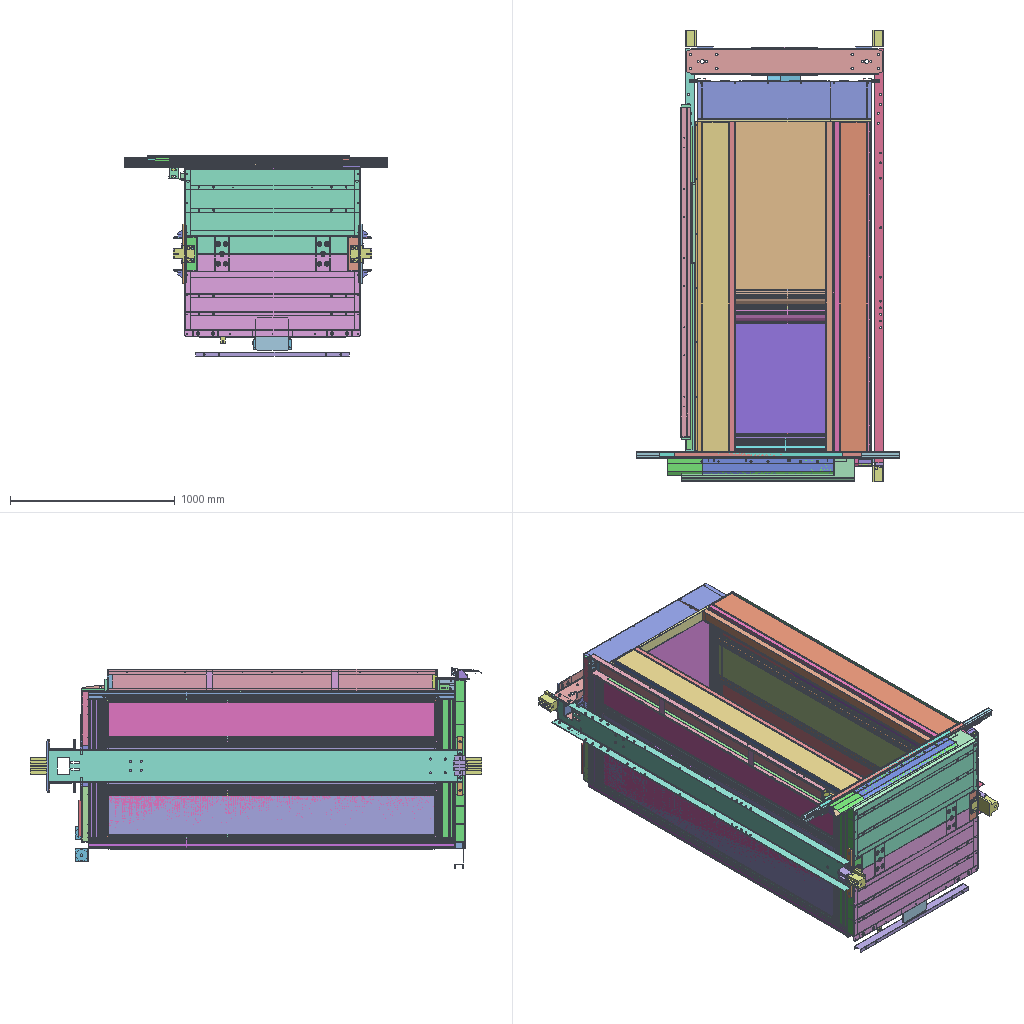Assembly | SolidWorks | 198 different items | 343 placed | box 1600 x 2739 x 1215 mm
Parts list (item | name | quantity | parent item):
1 | 25-2905 25-220S   常规梯专用电缆板A | x1 | in 145
2 | 25-2905 25-220S   轿顶简易盖板 | x1 | in 145
3 | 25-2905 25-220S   轿顶装饰板前 | x2 | in 145
4 | 25-2905 25-220S   轿顶装饰板后 | x2 | in 145
5 | 25-2905 25-220S  70地坎支架 | x1 | in 29
6 | 25-2905 25-220S  70地坎支架筋板 | x4 | in 29
7 | 25-2905 25-220S  L型支架 | x12 | in 135
8 | 25-2905 25-220S  U型支架 | x4 | in 131
9 | 25-2905 25-220S  歌拉瑞70旁开门地坎支架 | x1 | in 10
10 | 25-2905 25-220S  歌拉瑞70旁开门地坎支架焊件 (subassembly) | x1 | in 124
11 | 25-2905 25-220S  歌拉瑞70旁开门地坎支架筋板 | x4 | in 10
12 | 25-2905 25-220S  称重板 | x1 | in 142
13 | 25-2905 25-220S  背玻璃框（栅格板）（含扶手版） | x1 | in 135
14 | 25-2905 25-220S  轿底电缆固定板 | x1 | in 142
15 | 25-2905 25-220S  铝合金地坎(更新） | x1 | in 137
16 | 25-2905 25-220S 40地坎支架 | x1 | in 18
17 | 25-2905 25-220S 40地坎支架加筋 | x6 | in 18
18 | 25-2905 25-220S 40地坎支架焊件 (subassembly) | x1 | in 19
19 | 25-2905 25-220S 40地坎组件 (subassembly) | x1 | in 102
20 | 25-2905 25-220S 40护脚板 | x1 | in 19
21 | 25-2905 25-220S 40铝合金地坎 | x1 | in 19
22 | 25-2905 25-220S 60地坎护脚板 | x1 | in 26
23 | 25-2905 25-220S 60地坎支架 | x1 | in 24
24 | 25-2905 25-220S 60地坎支架焊件 (subassembly) | x1 | in 26
25 | 25-2905 25-220S 60地坎支架筋板 | x4 | in 24
26 | 25-2905 25-220S 60地坎支架组件 (subassembly) | x1 | in 102
27 | 25-2905 25-220S 60铝合金地坎 | x1 | in 26
28 | 25-2905 25-220S 70地坎(中分双折) | x1 | in 30
29 | 25-2905 25-220S 70地坎支架焊件(中分双折) (subassembly) | x1 | in 30
30 | 25-2905 25-220S 70地坎支架组件(中分双折) (subassembly) | x1 | in 102
31 | 25-2905 25-220S 70护脚板(中分双折) | x1 | in 30
32 | 25-2905 25-220S DD  吊顶 (subassembly) | x1 | in 137
33 | 25-2905 25-220S DD  外协吊顶 | x1 | in 32
34 | 25-2905 25-220S DD  星空顶A主板 | x1 | in 38
35 | 25-2905 25-220S DD  星空顶A客户确认图 (subassembly) | x1 | in 32
36 | 25-2905 25-220S DD  星空顶A封板 | x1 | in 38
37 | 25-2905 25-220S DD  星空顶A灯条框 | x1 | in 35
38 | 25-2905 25-220S DD  星空顶A焊件 (subassembly) | x1 | in 35
39 | 25-2905 25-220S DD  琉璃顶-内板 | x1 | in 42
40 | 25-2905 25-220S DD  琉璃顶-客户确认图 (subassembly) | x1 | in 32
41 | 25-2905 25-220S DD  琉璃顶-扩散板 | x1 | in 42
42 | 25-2905 25-220S DD  琉璃顶-灯罩框架 (subassembly) | x1 | in 40
43 | 25-2905 25-220S DD  琉璃顶-焊件总成 (subassembly) | x1 | in 40
44 | 25-2905 25-220S DD  琉璃顶-避让钣金 | x1 | in 43
45 | 25-2905 25-220S DD  琉璃顶-铝合金边框 | x1 | in 42
46 | 25-2905 25-220S DD  琉璃顶主板 | x1 | in 43
47 | 25-2905 25-220S DD  白顶-主板 | x1 | in 50
48 | 25-2905 25-220S DD  白顶-避让钣金 | x1 | in 50
49 | 25-2905 25-220S DD  白顶客户确认图 (subassembly) | x1 | in 32
50 | 25-2905 25-220S DD  白顶焊件总成 (subassembly) | x1 | in 49
51 | 25-2905 25-220S DD  白顶边框 | x1 | in 49
52 | 25-2905 25-220S DD-B1  白顶A主板 | x1 | in 56
53 | 25-2905 25-220S DD-B1  白顶A客户确认图 (subassembly) | x1 | in 32
54 | 25-2905 25-220S DD-B1  白顶A封板 | x1 | in 56
55 | 25-2905 25-220S DD-B1  白顶A灯条框 | x1 | in 53
56 | 25-2905 25-220S DD-B1  白顶A焊件 (subassembly) | x1 | in 53
57 | 25-2905 25-220S DD-X1  星空顶A主板 | x1 | in 61
58 | 25-2905 25-220S DD-X1  星空顶A客户确认图 (subassembly) | x1 | in 32
59 | 25-2905 25-220S DD-X1  星空顶A封板 | x1 | in 61
60 | 25-2905 25-220S DD-X1  星空顶A灯条框 | x1 | in 58
61 | 25-2905 25-220S DD-X1  星空顶A焊件 (subassembly) | x1 | in 58
62 | 25-2905 25-220S gyfb-75198(歌拉瑞专用风机) | x2 | in 137, 145
63 | 25-2905 25-220S 中立柱安装总成 (右侧） (subassembly) | x1 | in 131
64 | 25-2905 25-220S 中立柱安装总成 (左侧） (subassembly) | x1 | in 131
65 | 25-2905 25-220S 中间立柱COP外盖板 | x1 | in 64
66 | 25-2905 25-220S 中间立柱COP安装板 | x2 | in 64
67 | 25-2905 25-220S 中间立柱背板  (右侧） | x1 | in 63
68 | 25-2905 25-220S 中间立柱背板  (左侧） | x1 | in 64
69 | 25-2905 25-220S 中间立柱面板 (右侧） | x1 | in 63
70 | 25-2905 25-220S 中间立柱面板 (左侧） | x1 | in 64
71 | 25-2905 25-220S 侧前玻璃框 | x2 | in 135
72 | 25-2905 25-220S 侧后玻璃框 | x2 | in 135
73 | 25-2905 25-220S 侧玻璃框（HCS511) | x1 | in 135
74 | 25-2905 25-220S 侧筋板 | x22 | in 142
75 | 25-2905 25-220S 前壁右操纵箱加筋上（HOP029） | x1 | in 96
76 | 25-2905 25-220S 前壁右操纵箱加筋下（HOP029） | x1 | in 96
77 | 25-2905 25-220S 前壁左操纵箱加筋上（HOP029） | x1 | in 112
78 | 25-2905 25-220S 前壁左操纵箱加筋下（HOP029） | x1 | in 112
79 | 25-2905 25-220S 前壁操纵箱安装板（HOP029） | x2 | in 96, 112
80 | 25-2905 25-220S 反折DD-B1  白顶A主板 | x1 | in 82
81 | 25-2905 25-220S 反折DD-B1  白顶A封板 | x1 | in 82
82 | 25-2905 25-220S 反折DD-B1  白顶A焊件 (subassembly) | x1 | in 53
83 | 25-2905 25-220S 反折DD-X1  星空顶A主板 | x1 | in 85
84 | 25-2905 25-220S 反折DD-X1  星空顶A封板 | x1 | in 85
85 | 25-2905 25-220S 反折DD-X1  星空顶A焊件 (subassembly) | x1 | in 58
86 | 25-2905 25-220S 台阶螺钉 | x24 | in 63, 64
87 | 25-2905 25-220S 右前壁一体操纵箱 | x1 | in 137
88 | 25-2905 25-220S 右前壁下安装板 | x1 | in 93
89 | 25-2905 25-220S 右前壁主板 | x1 | in 93
90 | 25-2905 25-220S 右前壁常规加筋 | x1 | in 96
91 | 25-2905 25-220S 右前壁操纵箱加筋 | x2 | in 96
92 | 25-2905 25-220S 右前壁操纵箱加筋A | x1 | in 96
93 | 25-2905 25-220S 右前壁焊件 (subassembly) | x1 | in 96
94 | 25-2905 25-220S 右前壁盖板 | x1 | in 96
95 | 25-2905 25-220S 右前壁盖板（齐平盖板） | x1 | in 96
96 | 25-2905 25-220S 右前壁组件 (subassembly) | x1 | in 136
97 | 25-2905 25-220S 后玻璃框 | x1 | in 135
98 | 25-2905 25-220S 后筋板 | x6 | in 142
99 | 25-2905 25-220S 圆弧底板 | x2 | in 101
100 | 25-2905 25-220S 圆弧盖板 | x2 | in 101
101 | 25-2905 25-220S 圆弧盖板装配体 (subassembly) | x2 | in 135
102 | 25-2905 25-220S 地坎综合 (subassembly) | x1 | in 137
103 | 25-2905 25-220S 左前壁一体操纵箱 | x1 | in 137
104 | 25-2905 25-220S 左前壁下安装板 | x1 | in 109
105 | 25-2905 25-220S 左前壁主板 | x1 | in 109
106 | 25-2905 25-220S 左前壁常规加筋 | x1 | in 112
107 | 25-2905 25-220S 左前壁操纵箱加筋 | x2 | in 112
108 | 25-2905 25-220S 左前壁操纵箱加筋A | x1 | in 112
109 | 25-2905 25-220S 左前壁焊件 (subassembly) | x1 | in 112
110 | 25-2905 25-220S 左前壁盖板 | x1 | in 112
111 | 25-2905 25-220S 左前壁盖板（齐平盖板） | x1 | in 112
112 | 25-2905 25-220S 左前壁组件 (subassembly) | x1 | in 136
113 | 25-2905 25-220S 旁开门前壁主板 | x1 | in 117
114 | 25-2905 25-220S 旁开门前壁加筋 | x2 | in 117
115 | 25-2905 25-220S 旁开门前壁垫板 | x2 | in 118
116 | 25-2905 25-220S 旁开门前壁安装板 | x1 | in 117
117 | 25-2905 25-220S 旁开门前壁焊件 (subassembly) | x1 | in 118
118 | 25-2905 25-220S 旁开门前壁组件 (subassembly) | x1 | in 137
119 | 25-2905 25-220S 标准LOGO踏板 | x1 | in 137
120 | 25-2905 25-220S 横向加筋 | x2 | in 147
121 | 25-2905 25-220S 歌拉瑞-COP   (HOP027) | x3 | in 64, 96, 112
122 | 25-2905 25-220S 歌拉瑞-COP   (HOP029) | x3 | in 64, 96, 112
123 | 25-2905 25-220S 歌拉瑞70旁开门地坎 | x1 | in 124
124 | 25-2905 25-220S 歌拉瑞70旁开门地坎组件 (subassembly) | x1 | in 102
125 | 25-2905 25-220S 歌拉瑞70旁开门护脚板 | x1 | in 124
126 | 25-2905 25-220S 磁栅尺支架 | x2 | in 147
127 | 25-2905 25-220S 立柱面板加强型材 | x4 | in 63, 64
128 | 25-2905 25-220S 纵向加筋 | x2 | in 147
129 | 25-2905 25-220S 背玻璃框后壁扶手 | x1 | in 135
130 | 25-2905 25-220S 轿厢中立柱型材 | x4 | in 131
131 | 25-2905 25-220S 轿厢中立柱总成 (subassembly) | x1 | in 135
132 | 25-2905 25-220S 轿厢中立柱灯带 | x4 | in 131
133 | 25-2905 25-220S 轿厢中立柱灯带盖板 | x4 | in 131
134 | 25-2905 25-220S 轿厢型材框架 | x1 | in 135
135 | 25-2905 25-220S 轿厢型材框架A (subassembly) | x1 | in 136
136 | 25-2905 25-220S 轿厢总成 (subassembly) | x1 | in 137
137 | 25-2905 25-220S 轿厢总成A (subassembly) | x1 | -
138 | 25-2905 25-220S 轿底两侧加强筋 | x1 | in 142
139 | 25-2905 25-220S 轿底主板 | x1 | in 142
140 | 25-2905 25-220S 轿底加筋 | x6 | in 142
141 | 25-2905 25-220S 轿底横向加强筋 | x1 | in 142
142 | 25-2905 25-220S 轿底焊接总成 (subassembly) | x1 | in 143
143 | 25-2905 25-220S 轿底装配总成 (subassembly) | x1 | in 136
144 | 25-2905 25-220S 轿顶主板 | x1 | in 147
145 | 25-2905 25-220S 轿顶安装总成 (subassembly) | x1 | in 136
146 | 25-2905 25-220S 轿顶横向边梁 | x1 | in 147
147 | 25-2905 25-220S 轿顶焊接总成 (subassembly) | x1 | in 145
148 | 25-2905 25-220S 轿顶纵向边梁 | x1 | in 147
149 | 25-2905 25-220S 轿顶防晃支架 | x2 | in 147
150 | 25-2905 25-220S 门机支架 | x2 | in 147
151 | 25-2905 25-220S 门机支架A | x1 | in 147
152 | 25-2905 25-220S 门楣主板 | x1 | in 156
153 | 25-2905 25-220S 门楣加筋 | x1 | in 156
154 | 25-2905 25-220S 门楣加筋（门机门楣安装） | x1 | in 156
155 | 25-2905 25-220S 门楣安装件 (subassembly) | x1 | in 136
156 | 25-2905 25-220S 门楣焊件 (subassembly) | x1 | in 155
157 | 25-2905 25-220S 门楣盖板 | x1 | in 155
158 | 25-2905 25-220S 非标加筋中横 | x2 | in 147
159 | 25-2905 25-220S 非标加筋侧横 | x4 | in 147
160 | 25-2905 25-220S 非标加筋竖 | x2 | in 147
161 | 25-2905 25-220S-G 侧筋板A | x4 | in 171
162 | 25-2905 25-220S-G 侧筋板B | x1 | -
163 | 25-2905 25-220S-G 后筋板 | x6 | in 171
164 | 25-2905 25-220S-G 轿底两侧加强筋 | x1 | in 171
165 | 25-2905 25-220S-G 轿底中间加筋A | x2 | in 171
166 | 25-2905 25-220S-G 轿底中间加筋B | x4 | in 171
167 | 25-2905 25-220S-G 轿底主板 | x1 | in 171
168 | 25-2905 25-220S-G 轿底安装孔内加厚板 | x2 | in 171
169 | 25-2905 25-220S-G 轿底安装总成 (subassembly) | x1 | in 136
170 | 25-2905 25-220S-G 轿底横向加强筋 | x1 | in 171
171 | 25-2905 25-220S-G 轿底焊接总成 (subassembly) | x1 | in 169
172 | 25-2905 25-220S-G 轿底盖板 | x1 | in 169
173 | 25-2905 25-220S-G 轿底缓冲器加筋 | x2 | in 171
174 | 25-2905 GEH160 梁总成 (subassembly) | x1 | -
175 | 25-2905 GEH160上梁主板（3A646) | x2 | in 176
176 | 25-2905 GEH160上梁装配（3A654) (subassembly) | x1 | in 174
177 | 25-2905 GEH160导靴板（3A277) | x2 | in 176
178 | 25-2905 GEH160立梁主板（3B389) | x1 | in 182
179 | 25-2905 GEH160立梁安装板（3B384) | x1 | in 182
180 | 25-2905 GEH160立梁绳头上板（3B288) | x1 | in 176
181 | 25-2905 GEH160立梁绳头座（3B289) | x1 | in 176
182 | 25-2905 GEH160立梁装配（3B387) (subassembly) | x1 | in 174
183 | 25-2905 减震垫（BB011) | x1 | -
184 | 25-2905 外购A-1 电梯防晃卡板 | x4 | -
185 | 25-2905 导靴 | x2 | in 182, 198
186 | 25-2905 歌拉瑞 3Z159001导靴 | x4 | in 174
187 | 25-2905 镜向25-220S 侧玻璃框（HCS511) | x1 | in 135
188 | 25-2905 镜向25-220S 右前壁下安装板 | x1 | in 93
189 | 25-2905 镜向25-220S 左前壁下安装板 | x1 | in 109
190 | 25-2905 镜向25-220S 旁开门前壁安装板 | x1 | in 117
191 | 25-2905 镜向25-220S 轿底两侧加强筋 | x1 | in 142
192 | 25-2905 镜向25-220S 轿顶纵向边梁 | x1 | in 147
193 | 25-2905 镜向25-220S 门楣加筋 | x1 | in 156
194 | 25-2905 镜向25-220S-G 轿底两侧加强筋 | x1 | in 171
195 | hexagon weld nuts gb | x1 | -
196 | 镜向25-2905 GEH160立梁主板（3B266) | x1 | in 198
197 | 镜向25-2905 GEH160立梁安装板（3B265) | x1 | in 198
198 | 镜向25-2905 GEH160立梁装配（3B262) (subassembly) | x1 | in 174
Mates (type | each side: item.copy, entity, surface, feature):
In the top assembly
Coincident | assembly face | assembly face
Concentric | assembly face | assembly face
Coincident | 174.1 plane | assembly plane | 3 times
Coincident | 137.1 plane | assembly plane | 2 times
Width | 179.1 face plane 基体-法兰1 | 179.1 face plane 基体-法兰1 | 167.1 face plane 基体-法兰1 | 194.1 face plane 25-2905 25-220S-G 轿底两侧加强筋_镜向
Coincident | 178.1 face plane 基体-法兰1 | 184.1 face plane 凸台-拉伸1 | 2 times
Coincident | 149.1 face plane 边线-法兰1 | 184.1 face plane 基体-法兰1
In subassembly 174
Coincident | 174.2 face | 174.2 face
Concentric | 174.2 face | 174.2 face
Coincident | 176.1 plane | 174.2 plane | 2 times
Coincident | 182.1 plane | 174.2 plane
Coincident | 175.1 face plane 边线-法兰1 | 174.2 plane
Coincident | 175.1 face plane 边线-法兰1 | 178.2 face plane 基体-法兰1
Coincident | 177.1 face plane 基体-法兰1 | 186.1 face plane 凸台-拉伸1
Coincident | 174.2 plane | 186.1 plane
DistanceDim | 186.1 face plane 切除-拉伸1 | 178.2 face plane 基体-法兰1
Coincident | 186.1 face plane 切除-拉伸1 | 186.2 face plane 切除-拉伸1 | 2 times
DistanceDim | 186.2 face plane 凸台-拉伸1 | 178.2 face plane 基体-法兰1
Coincident | 186.1 plane | 174.2 plane
DistanceDim | 175.1 face plane 基体-法兰1 | 178.2 face plane 基体-法兰1
In subassembly 176
Coincident | 176.2 face | 176.2 face
Concentric | 176.2 face | 176.2 face
Coincident | 175.2 plane | 176.2 plane
Coincident | 175.2 face plane 边线-法兰1 | 176.2 plane
DistanceDim | 175.3 face plane 基体-法兰1 | 175.2 face plane 基体-法兰1
Coincident | 175.2 face plane 边线-法兰1 | 177.2 face plane 基体-法兰1
Coincident | 177.2 plane | 176.2 plane
DistanceDim | 177.2 plane | 175.3 face plane 基体-法兰1
Coincident | 181.1 plane | 176.2 plane | 2 times
Coincident | 175.2 face plane 边线-法兰1 | 181.1 face plane 边线-法兰2
Coincident | 180.1 plane | 176.2 plane | 2 times
Coincident | 175.3 face plane 边线-法兰1 | 180.1 face plane 基体-法兰1
In subassembly 182
Coincident | 182.2 face | 182.2 face
Concentric | 182.2 face | 182.2 face
Coincident | 178.3 plane | 182.2 plane
Coincident | 178.3 face plane 基体-法兰1 | 182.2 plane | 2 times
Coincident | 178.3 face plane 基体-法兰1 | 179.2 face plane 基体-法兰1 | 2 times
Coincident | 179.2 plane | 182.2 plane
Coincident | 178.3 face plane 基体-法兰1 | 185.1 face plane 凸台-拉伸1
DistanceDim | 185.1 face plane 凸台-拉伸1 | 178.3 face plane 基体-法兰1
In subassembly 137
Coincident | 137.2 face | 137.2 face
Concentric | 137.2 face | 137.2 face
Coincident | 136.1 plane | 137.2 plane | 3 times
DistanceDim | 21.1 face plane 凸台-拉伸1 | 134.1 face plane 25型材 25型材小立柱（最新）(1)
Coincident | 134.1 plane | 102.1 plane
Coincident | 139.1 face plane 基体-法兰1 | 103.1 face plane 镜向1
Coincident | 139.1 face plane 基体-法兰1 | 87.1 face plane 凸台-拉伸3
Coincident | 134.1 face plane 25型材 25型材小立柱（最新）(1) | 119.1 face plane 凸台-拉伸1 | 2 times
Coincident | 134.1 plane | 119.1 plane
Coincident | 21.1 face plane 凸台-拉伸1 | 15.1 face plane 凸台-拉伸1
Coincident | 16.1 face plane 基体-法兰1 | 15.1 face plane 凸台-拉伸1
Coincident | 15.1 plane | 137.2 plane
Coincident | 144.1 face plane 基体-法兰1 | 62.1 face plane 凸台-拉伸1
DistanceDim | 134.1 face plane 25型材 25型材小立柱（最新）(1) | 16.1 face plane 基体-法兰1
Coincident | 134.1 face plane 25型材 25型材小立柱（最新）(1) | 113.1 face plane 基体-法兰1
Coincident | 134.1 face plane 25型材 25型材小立柱（最新）(1) | 87.1 face plane 凸台-拉伸2
Coincident | 134.1 face plane 25型材 25型材小立柱（最新）(1) | 87.1 face plane 凸台-拉伸1
Coincident | 134.1 face plane 25型材 25型材小立柱（最新）(1) | 103.1 face plane 凸台-拉伸2
Coincident | 134.1 face plane 25型材 25型材小立柱（最新）(1) | 103.1 face plane 凸台-拉伸1
DistanceDim | 33.1 face plane 凸台-拉伸1 | 134.1 face plane 25轿厢 GC505&506(1) | 2 times
Coincident | 144.1 face plane 基体-法兰1 | 33.1 face plane 凸台-拉伸1
In subassembly 136
Coincident | 136.2 face | 136.2 face
Concentric | 136.2 face | 136.2 face
Coincident | 135.1 plane | 136.2 plane | 3 times
Coincident | 145.1 plane | 136.2 plane | 2 times
Coincident | 134.2 face plane  D:\xxxxxx\xxxx\xxxx\xxxx\xxxx\xxxxxxxxxxxxx | 144.2 face plane 基体-法兰1
Coincident | 155.1 plane | 136.2 plane
Coincident | 144.2 face plane 边线-法兰2 | 152.1 face plane 边线-法兰5
Coincident | 143.1 plane | 136.2 plane | 2 times
Coincident | 134.2 face plane  D:\xxxxxx\xxxx\xxxx\xxxx\xxxx\xxxxxxxxxxxxx | 139.2 face plane 基体-法兰1
Coincident | 139.2 face plane 基体-法兰1 | 189.1 face plane 25-2905 25-220S 左前壁下安装板_镜向
Coincident | 171.1 plane | 136.2 plane
Coincident | 134.2 face plane 25轿厢 GC503(1) | 167.2 face plane 基体-法兰1
Coincident | 169.1 plane | 136.2 plane
Coincident | 134.2 face plane 25型材 25型材小立柱（最新）(1) | 88.1 face plane 基体-法兰1
Coincident | 134.2 face plane 25型材 25型材小立柱（最新）(1) | 152.1 face plane 基体-法兰1
Coincident | 134.2 face plane 25型材 25型材小立柱（最新）(1) | 105.1 face plane 基体-法兰1 | 2 times
Coincident | 134.2 face plane 25型材 25型材小立柱（最新）(1) | 89.1 face plane 基体-法兰1 | 2 times
In subassembly 135
Coincident | 135.2 face | 135.2 face
Concentric | 135.2 face | 135.2 face
Coincident | 134.3 plane | 135.2 plane | 3 times
Coincident | 131.1 plane | 135.2 plane | 2 times
Coincident | 134.3 face plane 25轿厢 GC503(1) | 130.1 face plane 凸台-拉伸1
Width | 7.1 face plane 基体-法兰1 | 7.1 face plane 基体-法兰1 | 134.3 face plane 25轿厢 GC503(1) | 134.3 face plane 25轿厢 GC503(1)
Coincident | 134.3 face plane 25轿厢 GC503(1) | 7.1 face plane 基体-法兰1
Coincident | 134.3 face plane  D:\xxxxxx\xxxx\xxxx\xxxx\xxxx\xxxxxxxxxxxxx | 7.1 face plane 基体-法兰1
Coincident | 134.3 face plane  D:\xxxxxx\xxxx\xxxx\xxxx\xxxx\xxxxxxxxxxxxx | 7.2 face plane 基体-法兰1
Parallel | 7.2 edge | 7.1 face plane 基体-法兰1
Coincident | 7.1 edge | 7.2 face plane 基体-法兰1
Coincident | 134.3 face plane 25轿厢 GC505&506(1) | 7.2 face plane 基体-法兰1
Coincident | 7.1 face plane 基体-法兰1 | 7.3 face plane 基体-法兰1
Coincident | 134.3 face plane  D:\xxxxxx\xxxx\xxxx\xxxx\xxxx\xxxxxxxxxxxxx | 7.3 face plane 基体-法兰1
Width | 7.3 face plane 基体-法兰1 | 7.3 face plane 基体-法兰1 | 134.3 face plane 25轿厢 GC503(1) | 134.3 face plane 25轿厢 GC503(1)
Coincident | 134.3 face plane 25轿厢 GC505&506(1) | 7.4 face plane 基体-法兰1
Coincident | 134.3 face plane  D:\xxxxxx\xxxx\xxxx\xxxx\xxxx\xxxxxxxxxxxxx | 7.4 face plane 基体-法兰1
Coincident | 7.3 face plane 基体-法兰1 | 7.4 edge
Coincident | 97.1 face plane  D:\xxxxxx\xx\xxxx\xxxx\xxxxxx\xxx\xxxxxxxxxxxx | 129.1 face plane  D:\xxxxxx\xx\xxxx\xxxx\xxxxxx\xxx\xxxxxxxxxxxx | 3 times
Coincident | 97.1 plane | 135.2 plane
Coincident | 134.3 face plane 25轿厢 GC503(1) | 97.1 face plane  D:\xxxxxx\xx\xxxx\xxxx\xxxxxx\xxx\xxxxxxxxxxxx | 2 times
Coincident | 134.3 face plane 25轿厢 GC503(1) | 72.1 face plane  D:\xxxxxx\xx\xxxx\xxxx\xxxxxx\xxx\xxxxxxxxxxxx | 2 times
Coincident | 134.3 face plane 25轿厢 GC503(1) | 73.1 face plane  D:\xxxxxx\xx\xxxx\xxxx\xxxxxx\xxx\xxxxxxxxxxxx | 2 times
Coincident | 134.3 face plane 25轿厢 GC503(1) | 71.1 face plane  D:\xxxxxx\xx\xxxx\xxxx\xxxxxx\xxx\xxxxxxxxxxxx | 2 times
DistanceDim | 134.3 edge | 72.1 face plane  D:\xxxxxx\xx\xxxx\xxxx\xxxxxx\xxx\xxxxxxxxxxxx
DistanceDim | 134.3 face plane  D:\xxxxxx\xxxx\xxxx\xxxx\xxxx\xxxxxxxxxxxxx | 73.1 face plane  D:\xxxxxx\xx\xxxx\xxxx\xxxxxx\xxx\xxxxxxxxxxxx
Coincident | 134.3 face plane  D:\xxxxxx\xxxx\xxxx\xxxx\xxxx\xxxxxxxxxxxxx | 99.1 face plane 凸台-拉伸1
Width | 99.1 face plane 凸台-拉伸1 | 99.1 face plane 凸台-拉伸1 | 134.3 face plane  D:\xxxxxx\xxxx\xxxx\xxxx\xxxx\xxxxxxxxxxxxx | 134.3 face plane  D:\xxxxxx\xxxx\xxxx\xxxx\xxxx\xxxxxxxxxxxxx
Coincident | 134.3 face plane  D:\xxxxxx\xxxx\xxxx\xxxx\xxxx\xxxxxxxxxxxxx | 100.1 face plane 凸台-拉伸1
DistanceDim | 130.1 face plane 凸台-拉伸1 | 71.1 edge
Coincident | 134.3 face plane 25轿厢 GC503(1) | 7.5 face plane 基体-法兰1
Coincident | 134.3 face plane 25型材 25型材小立柱（最新）(1) | 7.5 face plane 基体-法兰1
Coincident | 7.3 face plane 基体-法兰1 | 7.5 face plane 基体-法兰1
Coincident | 7.5 face plane 基体-法兰1 | 7.6 face plane 基体-法兰1 | 2 times
Coincident | 134.3 face plane 25轿厢 GC505&506(1) | 7.6 face plane 基体-法兰1
Coincident | 97.1 face plane  D:\xxxxxx\xx\xxxx\xxxx\xxxxxx\xxx\xxxxxxxxxxxx | 13.1 face plane  D:\xxxxxx\xx\xxxx\xxxx\xxxxxx\xxx\xxxxxxxxxxxx | 3 times
In subassembly 101
Coincident | 101.1 face | 101.1 face
Concentric | 101.1 face | 101.1 face
Coincident | 99.2 plane | 101.1 plane | 3 times
Coincident | 100.2 plane | 101.1 plane | 3 times
In subassembly 131
Coincident | 131.2 face | 131.2 face
Concentric | 131.2 face | 131.2 face
Parallel | 130.2 face plane 凸台-拉伸1 | 131.2 plane | 2 times
Coincident | 130.2 face plane 凸台-拉伸1 | 132.1 face plane 凸台-拉伸1 | 2 times
Coincident | 130.2 plane | 131.2 plane
Coincident | 132.1 plane | 131.2 plane
DistanceDim | 132.1 face plane 凸台-拉伸1 | 133.1 face plane 凸台-拉伸1
Coincident | 133.1 plane | 131.2 plane
Coincident | 132.1 face plane 凸台-拉伸1 | 133.1 edge
Coincident | 130.2 face plane 凸台-拉伸1 | 131.2 select_type:10 | 2 times
Coincident | 64.1 plane | 131.2 plane | 2 times
Coincident | 68.1 face plane 基体-法兰1 | 130.3 face plane 凸台-拉伸1
Coincident | 130.4 face plane 凸台-拉伸1 | 67.1 face plane 基体-法兰1
Coincident | 8.1 plane | 131.2 plane
DistanceDim | 68.1 face plane 基体-法兰1 | 8.1 face plane 基体-法兰1
DistanceDim | 8.1 face plane 基体-法兰1 | 130.3 face plane 凸台-拉伸1
Coincident | 8.2 plane | 131.2 plane
Coincident | 8.1 face plane 基体-法兰1 | 8.2 face plane 基体-法兰1
DistanceDim | 130.2 face plane 凸台-拉伸1 | 8.2 face plane 基体-法兰1
Coincident | 63.1 plane | 131.2 plane | 2 times
In subassembly 64
Coincident | 64.2 face | 64.2 face
Concentric | 64.2 face | 64.2 face
Coincident | 68.2 plane | 64.2 plane | 2 times
Coincident | 68.2 face plane 基体-法兰1 | 64.2 plane
Coincident | 70.1 plane | 64.2 plane | 2 times
Concentric | 68.2 face cylinder 切除-拉伸2 | 70.1 face cylinder 切除-拉伸2
Coincident | 70.1 face plane 基体-法兰1 | 66.1 face plane 基体-法兰1
Coincident | 70.1 plane | 66.1 plane
Coincident | 70.1 face plane 基体-法兰1 | 127.1 face plane 拉伸-薄壁1 | 2 times
Coincident | 127.1 plane | 64.2 plane
Concentric | 68.2 face cylinder 切除-拉伸2 | 86.1 face cylinder 凸台-拉伸3
Coincident | 68.2 face plane 基体-法兰1 | 86.1 face plane 凸台-拉伸2
Concentric | 68.2 face cylinder 切除-拉伸2 | 86.2 face cylinder 凸台-拉伸2
Coincident | 68.2 face plane 基体-法兰1 | 86.2 face plane 凸台-拉伸2
Concentric | 68.2 face cylinder 切除-拉伸2 | 86.3 face cylinder 凸台-拉伸2
Coincident | 68.2 face plane 基体-法兰1 | 86.3 face plane 凸台-拉伸2
Concentric | 68.2 face cylinder 切除-拉伸2 | 86.4 face cylinder 凸台-拉伸2
Coincident | 68.2 face plane 基体-法兰1 | 86.4 face plane 凸台-拉伸2
Concentric | 68.2 face cylinder 切除-拉伸2 | 86.5 face cylinder 凸台-拉伸2
Coincident | 68.2 face plane 基体-法兰1 | 86.5 face plane 凸台-拉伸2
Concentric | 68.2 face cylinder 切除-拉伸2 | 86.6 face cylinder 凸台-拉伸2
Coincident | 68.2 face plane 基体-法兰1 | 86.6 face plane 凸台-拉伸2
Coincident | 121.1 plane | 64.2 plane | 2 times
Coincident | 70.1 face plane 基体-法兰1 | 121.1 face plane 凸台-拉伸1
Coincident | 65.1 plane | 64.2 plane
Coincident | 65.1 plane | 121.1 plane
Coincident | 68.2 face plane 基体-法兰1 | 65.1 face plane 边线-法兰2
Coincident | 122.1 plane | 64.2 plane | 2 times
Coincident | 70.1 face plane 基体-法兰1 | 122.1 face plane 凸台-拉伸1
DistanceDim | 66.1 face plane 基体-法兰1 | 68.2 face plane 基体-法兰1
In subassembly 63
Coincident | 63.2 face | 63.2 face
Concentric | 63.2 face | 63.2 face
Coincident | 67.2 plane | 63.2 plane | 2 times
Coincident | 67.2 face plane 基体-法兰1 | 63.2 plane
Coincident | 69.1 plane | 63.2 plane | 2 times
Concentric | 67.2 face cylinder 切除-拉伸2 | 69.1 face cylinder 切除-拉伸2
Coincident | 69.1 face plane 基体-法兰1 | 127.1 face plane 拉伸-薄壁1 | 2 times
Coincident | 127.1 plane | 63.2 plane
Concentric | 67.2 face cylinder 切除-拉伸2 | 86.1 face cylinder 凸台-拉伸3
Coincident | 67.2 face plane 基体-法兰1 | 86.1 face plane 凸台-拉伸2
Concentric | 67.2 face cylinder 切除-拉伸2 | 86.2 face cylinder 凸台-拉伸2
Coincident | 67.2 face plane 基体-法兰1 | 86.2 face plane 凸台-拉伸2
Concentric | 67.2 face cylinder 切除-拉伸2 | 86.3 face cylinder 凸台-拉伸2
Coincident | 67.2 face plane 基体-法兰1 | 86.3 face plane 凸台-拉伸2
Concentric | 67.2 face cylinder 切除-拉伸2 | 86.4 face cylinder 凸台-拉伸2
Coincident | 67.2 face plane 基体-法兰1 | 86.4 face plane 凸台-拉伸2
Concentric | 67.2 face cylinder 切除-拉伸2 | 86.5 face cylinder 凸台-拉伸2
Coincident | 67.2 face plane 基体-法兰1 | 86.5 face plane 凸台-拉伸2
Concentric | 67.2 face cylinder 切除-拉伸2 | 86.6 face cylinder 凸台-拉伸2
Coincident | 67.2 face plane 基体-法兰1 | 86.6 face plane 凸台-拉伸2
In subassembly 169
Coincident | 169.2 face | 169.2 face
Concentric | 169.2 face | 169.2 face
Coincident | 171.2 plane | 169.2 plane | 3 times
Coincident | 170.1 face plane 基体-法兰1 | 172.1 face plane 基体-法兰1
Coincident | 172.1 plane | 169.2 plane | 2 times
In subassembly 171
Coincident | 171.3 face | 171.3 face
Concentric | 171.3 face | 171.3 face
Coincident | 167.3 plane | 171.3 plane | 3 times
Coincident | 170.2 plane | 171.3 plane
Coincident | 167.3 face plane 基体-法兰1 | 170.2 face plane 基体-法兰1 | 2 times
Coincident | 167.3 face plane 基体-法兰1 | 166.1 face plane 基体-法兰1
Coincident | 166.1 plane | 171.3 plane
Coincident | 170.2 face plane 基体-法兰1 | 163.1 face plane 凸台-拉伸1 | 2 times
Coincident | 170.2 face plane 基体-法兰1 | 163.2 face plane 凸台-拉伸1 | 2 times
DistanceDim | 170.2 face plane 基体-法兰1 | 163.2 face plane 凸台-拉伸1
DistanceDim | 171.3 plane | 163.1 face plane 凸台-拉伸1
Coincident | 167.3 face plane 基体-法兰1 | 164.1 face plane 基体-法兰1 | 2 times
Coincident | 170.2 face plane 基体-法兰1 | 164.1 face plane 基体-法兰1
Coincident | 167.3 face plane 基体-法兰1 | 165.1 face plane 基体-法兰1
Coincident | 165.1 plane | 171.3 plane
Coincident | 167.3 face plane 基体-法兰1 | 173.1 face plane 边线-法兰1
Coincident | 173.1 plane | 171.3 plane
DistanceDim | 173.1 plane | 164.1 face plane 基体-法兰1
Coincident | 167.3 face plane 基体-法兰1 | 166.2 face plane 基体-法兰1
Coincident | 166.2 plane | 171.3 plane
Coincident | 164.1 face plane 基体-法兰1 | 168.1 face plane 基体-法兰1
Coincident | 168.1 plane | 171.3 plane
Width | 164.1 face plane 基体-法兰1 | 164.1 face plane 基体-法兰1 | 168.1 face plane 基体-法兰1 | 168.1 face plane 基体-法兰1
Coincident | 164.1 face plane 基体-法兰1 | 161.1 face plane 基体-法兰1 | 2 times
Coincident | 167.3 face plane 基体-法兰1 | 166.3 face plane 基体-法兰1
Coincident | 166.3 plane | 171.3 plane
Coincident | 167.3 face plane 基体-法兰1 | 166.4 face plane 基体-法兰1
Coincident | 166.4 plane | 171.3 plane
DistanceDim | 161.1 face plane 基体-法兰1 | 161.2 face plane 基体-法兰1
Coincident | 165.1 face plane 基体-法兰1 | 173.2 face plane 基体-法兰1
DistanceDim | 170.2 face plane 基体-法兰1 | 166.1 face plane 基体-法兰1
DistanceDim | 166.4 face plane 基体-法兰1 | 165.2 face plane 基体-法兰1
DistanceDim | 166.2 face plane 基体-法兰1 | 167.3 face plane 基体-法兰1
DistanceDim | 165.1 face plane 基体-法兰1 | 166.3 face plane 基体-法兰1
In subassembly 145
Coincident | 145.2 face | 145.2 face
Concentric | 145.2 face | 145.2 face
Coincident | 147.1 plane | 145.2 plane | 2 times
Coincident | 144.3 face plane 基体-法兰1 | 145.2 plane
Coincident | 2.1 plane | 145.2 plane | 2 times
Coincident | 146.1 face plane 基体-法兰1 | 2.1 face plane 基体-法兰1
Coincident | 2.1 face plane 基体-法兰1 | 1.1 face plane 基体-法兰1
Slot | 1.1 face cylinder 切除-拉伸1 | 146.1 face cylinder 切除-拉伸5
Parallel | 146.1 face plane 基体-法兰1 | 1.1 face plane 基体-法兰1
Coincident | 148.1 face plane 基体-法兰1 | 4.1 face plane 边线-法兰1
Coincident | 146.1 face plane 基体-法兰1 | 4.1 face plane 基体-法兰1 | 2 times
Coincident | 148.1 face plane 基体-法兰1 | 3.1 face plane 边线-法兰1
Coincident | 144.3 face plane 边线-法兰1 | 3.1 face plane 基体-法兰1 | 2 times
Coincident | 144.3 face plane 基体-法兰1 | 62.1 face plane 凸台-拉伸1
Coincident | 144.3 face plane 基体-法兰1 | 62.2 face
Concentric | 144.3 select_type:24 | 62.2 face
Parallel | 148.1 face plane 基体-法兰1 | 62.2 face
Concentric | 144.3 select_type:24 | 62.1 face cylinder 切除-拉伸3 | 2 times
In subassembly 147
Coincident | 147.2 face | 147.2 face
Concentric | 147.2 face | 147.2 face
Coincident | 144.4 plane | 147.2 plane | 2 times
Coincident | 144.4 face plane 基体-法兰1 | 147.2 plane
Coincident | 144.4 face plane 基体-法兰1 | 146.2 face plane 基体-法兰1 | 2 times
Coincident | 146.2 plane | 147.2 plane
Coincident | 144.4 face plane 基体-法兰1 | 148.2 face plane 基体-法兰1 | 2 times
Coincident | 146.2 face plane 基体-法兰1 | 148.2 face plane 基体-法兰1
Coincident | 144.4 face plane 基体-法兰1 | 150.1 face plane 基体-法兰1
Coincident | 150.1 plane | 147.2 plane
DistanceDim | 150.1 face plane 基体-法兰1 | 144.4 face plane 边线-法兰1
Coincident | 148.2 face plane 基体-法兰1 | 149.2 face plane 基体-法兰1
Coincident | 148.2 face plane 基体-法兰1 | 149.2 face plane 边线-法兰1
Coincident | 144.4 face plane 基体-法兰1 | 120.1 face plane 基体-法兰1
Coincident | 120.1 plane | 147.2 plane
Coincident | 144.4 face plane 基体-法兰1 | 128.1 face plane 基体-法兰1
Coincident | 120.1 face plane 基体-法兰1 | 128.1 face plane 基体-法兰1
Coincident | 120.1 plane | 128.1 plane
Coincident | 144.4 face plane 基体-法兰1 | 120.2 face plane 基体-法兰1
Coincident | 128.2 face plane 基体-法兰1 | 120.2 face plane 基体-法兰1
Coincident | 120.2 plane | 147.2 plane
DistanceDim | 120.1 face plane 基体-法兰1 | 146.2 face plane 基体-法兰1
Coincident | 148.2 plane | 149.2 plane
Coincident | 148.2 face plane 基体-法兰1 | 126.1 face plane 基体-法兰1 | 2 times
Coincident | 150.2 face plane 基体-法兰1 | 151.1 face plane 基体-法兰1
Coincident | 144.4 face plane 基体-法兰1 | 151.1 face plane 基体-法兰1
Coincident | 151.1 plane | 147.2 plane
DistanceDim | 146.2 face plane 基体-法兰1 | 126.1 face plane 基体-法兰1
Coincident | 144.4 face plane 基体-法兰1 | 160.1 face plane 基体-法兰1
Coincident | 150.2 face plane 基体-法兰1 | 160.1 face plane 基体-法兰1
Coincident | 144.4 face plane 基体-法兰1 | 158.1 face plane 基体-法兰1
Coincident | 158.1 plane | 147.2 plane
Coincident | 160.1 plane | 158.1 plane
Coincident | 144.4 face plane 基体-法兰1 | 159.1 face plane 基体-法兰1
Coincident | 160.1 face plane 基体-法兰1 | 159.1 face plane 基体-法兰1
Coincident | 158.1 face plane 基体-法兰1 | 159.1 face plane 基体-法兰1
Coincident | 148.2 face plane 基体-法兰1 | 159.1 face plane 基体-法兰1
Coincident | 144.4 face plane 基体-法兰1 | 159.2 face plane 基体-法兰1
Coincident | 158.1 face plane 基体-法兰1 | 159.2 face plane 基体-法兰1
Coincident | 160.2 face plane 基体-法兰1 | 159.2 face plane 基体-法兰1
In subassembly 155
Coincident | 155.2 face | 155.2 face
Concentric | 155.2 face | 155.2 face
Coincident | 156.1 plane | 155.2 plane | 3 times
Coincident | 157.1 plane | 155.2 plane
DistanceDim | 157.1 face plane 基体-法兰1 | 193.1 face plane 25-2905 25-220S 门楣加筋_镜向
DistanceDim | 193.1 face plane 25-2905 25-220S 门楣加筋_镜向 | 157.1 face plane 基体-法兰1
In subassembly 156
Coincident | 156.2 face | 156.2 face
Concentric | 156.2 face | 156.2 face
Coincident | 152.2 plane | 156.2 plane
Coincident | 152.2 face plane 基体-法兰1 | 156.2 plane | 2 times
Coincident | 152.2 face plane 基体-法兰1 | 153.1 face plane 边线-法兰1
Coincident | 152.2 face plane 基体-法兰1 | 153.1 face plane 边线-法兰2 | 2 times
Coincident | 152.2 face plane 基体-法兰1 | 154.1 face plane 边线-法兰1
Coincident | 152.2 face plane 基体-法兰1 | 154.1 face plane 边线-法兰2
In subassembly 112
Coincident | 112.1 face | 112.1 face
Concentric | 112.1 face | 112.1 face
Coincident | 109.1 plane | 112.1 plane | 3 times
Coincident | 110.1 plane | 112.1 plane
Coincident | 105.2 face plane 基体-法兰1 | 106.1 face plane 边线-法兰1
Coincident | 106.1 plane | 112.1 plane | 2 times
Coincident | 105.2 face plane 基体-法兰1 | 107.1 face plane 基体-法兰1
Coincident | 107.1 plane | 112.1 plane
Coincident | 105.2 face plane 基体-法兰1 | 108.1 face plane 基体-法兰1
Coincident | 107.1 plane | 108.1 plane
Coincident | 105.2 face plane 基体-法兰1 | 108.1 face plane 边线-法兰1
Coincident | 111.1 plane | 112.1 plane
Coincident | 104.1 plane | 111.1 plane
Coincident | 105.2 face plane 基体-法兰1 | 111.1 face plane 基体-法兰1
Coincident | 105.2 plane | 121.1 plane | 2 times
Coincident | 105.2 plane | 122.1 plane | 2 times
Coincident | 105.2 face plane 基体-法兰1 | 121.1 face plane 凸台-拉伸1
Coincident | 105.2 face plane 基体-法兰1 | 122.1 face plane 凸台-拉伸1
Coincident | 107.1 face plane 基体-法兰1 | 121.1 face plane 凸台-拉伸2
Coincident | 105.2 face plane 基体-法兰1 | 79.1 face plane 边线-法兰2
Coincident | 122.1 plane | 79.1 plane | 2 times
Coincident | 105.2 face plane 基体-法兰1 | 78.1 face plane 边线-法兰1
DistanceDim | 78.1 face plane 基体-法兰1 | 189.2 face plane 25-2905 25-220S 左前壁下安装板_镜向
Coincident | 78.1 plane | 112.1 plane
Coincident | 105.2 face plane 基体-法兰1 | 77.1 face plane 边线-法兰1
Coincident | 78.1 face plane 基体-法兰1 | 77.1 face plane 基体-法兰1
DistanceDim | 104.1 face plane 边线-法兰3 | 77.1 face plane 边线-法兰1
In subassembly 109
Coincident | 109.2 face | 109.2 face
Concentric | 109.2 face | 109.2 face
Coincident | 105.3 plane | 109.2 plane | 2 times
Coincident | 105.3 face plane 基体-法兰1 | 109.2 plane
Coincident | 104.2 plane | 109.2 plane | 2 times
Coincident | 105.3 face plane 基体-法兰1 | 104.2 face plane 基体-法兰1
In subassembly 96
Coincident | 96.1 face | 96.1 face
Concentric | 96.1 face | 96.1 face
Coincident | 93.1 plane | 96.1 plane | 3 times
Coincident | 94.1 plane | 96.1 plane
DistanceDim | 89.2 face plane 边线-法兰1 | 94.1 face plane 基体-法兰1
DistanceDim | 89.2 face plane 边线-法兰2 | 94.1 face plane 基体-法兰1
Coincident | 89.2 face plane 基体-法兰1 | 90.1 face plane 边线-法兰1
Coincident | 90.1 plane | 96.1 plane | 2 times
Coincident | 89.2 face plane 基体-法兰1 | 91.1 face plane 基体-法兰1
Coincident | 91.1 plane | 96.1 plane
Coincident | 89.2 face plane 基体-法兰1 | 92.1 face plane 基体-法兰1
Coincident | 91.1 plane | 92.1 plane
Coincident | 89.2 face plane 基体-法兰1 | 92.1 face plane 边线-法兰1
Coincident | 95.1 plane | 96.1 plane
Coincident | 88.2 plane | 95.1 plane
Coincident | 89.2 face plane 基体-法兰1 | 95.1 face plane 基体-法兰1
Coincident | 76.1 face plane 基体-法兰1 | 75.1 face plane 基体-法兰1 | 2 times
Coincident | 89.2 plane | 121.1 plane | 2 times
Coincident | 89.2 face plane 基体-法兰1 | 121.1 face plane 凸台-拉伸1
Coincident | 91.1 face plane 基体-法兰1 | 121.1 face plane 凸台-拉伸2
Coincident | 89.2 plane | 122.1 plane | 2 times
Coincident | 89.2 face plane 基体-法兰1 | 122.1 face plane 凸台-拉伸1
Coincident | 89.2 face plane 基体-法兰1 | 79.1 face plane 边线-法兰2
Coincident | 89.2 plane | 79.1 plane | 2 times
Coincident | 89.2 face plane 基体-法兰1 | 76.1 face plane 边线-法兰1
Coincident | 76.1 plane | 96.1 plane
DistanceDim | 76.1 face plane 基体-法兰1 | 88.2 face plane 边线-法兰3
Coincident | 89.2 face plane 基体-法兰1 | 75.1 face plane 边线-法兰1
DistanceDim | 188.1 face plane 25-2905 25-220S 右前壁下安装板_镜向 | 75.1 face plane 基体-法兰1
In subassembly 93
Coincident | 93.2 face | 93.2 face
Concentric | 93.2 face | 93.2 face
Coincident | 89.3 plane | 93.2 plane | 2 times
Coincident | 89.3 face plane 基体-法兰1 | 93.2 plane
Coincident | 88.3 plane | 93.2 plane | 2 times
Coincident | 89.3 face plane 基体-法兰1 | 88.3 face plane 基体-法兰1
In subassembly 143
Coincident | 143.2 face | 143.2 face
Concentric | 143.2 face | 143.2 face
Coincident | 142.1 plane | 143.2 plane | 3 times
In subassembly 142
Coincident | 142.2 face | 142.2 face
Concentric | 142.2 face | 142.2 face
Coincident | 139.3 plane | 142.2 plane | 3 times
Coincident | 141.1 plane | 142.2 plane
Coincident | 139.3 face plane 基体-法兰1 | 141.1 face plane 基体-法兰1 | 2 times
Coincident | 139.3 face plane 基体-法兰1 | 138.1 face plane 基体-法兰1 | 3 times
Coincident | 139.3 face plane 基体-法兰1 | 140.1 face plane 基体-法兰1
Coincident | 140.1 plane | 142.2 plane
DistanceDim | 140.1 face plane 基体-法兰1 | 139.3 face plane 基体-法兰1
Coincident | 141.1 face plane 基体-法兰1 | 98.1 face plane 凸台-拉伸1 | 2 times
Coincident | 141.1 face plane 基体-法兰1 | 98.2 face plane 凸台-拉伸1 | 2 times
DistanceDim | 141.1 face plane 基体-法兰1 | 98.2 face plane 凸台-拉伸1
DistanceDim | 142.2 plane | 98.1 face plane 凸台-拉伸1
Coincident | 138.1 face plane 基体-法兰1 | 74.1 face plane 基体-法兰1
DistanceDim | 138.1 face plane 基体-法兰1 | 74.1 face plane 基体-法兰1
DistanceDim | 74.1 face plane 基体-法兰1 | 139.3 face plane 基体-法兰1
Coincident | 74.1 face plane 基体-法兰1 | 74.2 face plane 基体-法兰1
Coincident | 138.1 face plane 基体-法兰1 | 74.2 face plane 基体-法兰1
DistanceDim | 74.2 face plane 基体-法兰1 | 139.3 face plane 基体-法兰1
Coincident | 138.1 face plane 基体-法兰1 | 74.3 face plane 基体-法兰1
Coincident | 74.1 face plane 基体-法兰1 | 74.3 face plane 基体-法兰1
DistanceDim | 142.2 plane | 74.3 face plane 基体-法兰1
Coincident | 141.1 face plane 基体-法兰1 | 12.1 face plane 凸台-拉伸1
Coincident | 12.1 plane | 142.2 plane
Coincident | 141.1 face plane 基体-法兰1 | 14.1 face plane 凸台-拉伸1
DistanceDim | 14.1 plane | 142.2 plane
Width | 14.1 face plane 凸台-拉伸1 | 14.1 face plane 凸台-拉伸1 | 141.1 face plane 基体-法兰1 | 141.1 face plane 基体-法兰1
Width | 12.1 face plane 凸台-拉伸1 | 12.1 face plane 凸台-拉伸1 | 141.1 face plane 基体-法兰1 | 141.1 face plane 基体-法兰1
In subassembly 102
Coincident | 102.2 face | 102.2 face
Concentric | 102.2 face | 102.2 face
Coincident | 19.1 plane | 102.2 plane | 3 times
Coincident | 16.2 face plane 基体-法兰1 | 5.1 face plane 基体-法兰1
Coincident | 21.2 face plane 凸台-拉伸1 | 28.1 face plane 凸台-拉伸1
Coincident | 30.1 plane | 102.2 plane
Coincident | 26.1 plane | 102.2 plane
Coincident | 16.2 face plane 基体-法兰1 | 23.1 face plane 基体-法兰1
Coincident | 21.2 face plane 凸台-拉伸1 | 27.1 face plane 凸台-拉伸1
Coincident | 16.2 face plane 基体-法兰1 | 9.1 face plane 基体-法兰1
Coincident | 21.2 face plane 凸台-拉伸1 | 123.1 face plane 凸台-拉伸1
In subassembly 19
Coincident | 19.2 face | 19.2 face
Concentric | 19.2 face | 19.2 face
Coincident | 18.1 plane | 19.2 plane | 3 times
Coincident | 16.3 face plane 基体-法兰1 | 21.3 face plane 凸台-拉伸1 | 2 times
Coincident | 21.3 plane | 19.2 plane
Coincident | 16.3 face plane 基体-法兰1 | 20.1 face plane 基体-法兰1
Coincident | 20.1 plane | 19.2 plane
Coincident | 21.3 face plane 凸台-拉伸1 | 20.1 face plane 基体-法兰1
In subassembly 18
Coincident | 18.2 face | 18.2 face
Concentric | 18.2 face | 18.2 face
Coincident | 16.4 plane | 18.2 plane | 2 times
Coincident | 16.4 face plane 基体-法兰1 | 18.2 plane
Coincident | 16.4 face plane 基体-法兰1 | 17.1 face plane 凸台-拉伸1 | 2 times
DistanceDim | 16.4 face plane 基体-法兰1 | 17.1 edge
In subassembly 26
Coincident | 26.2 face | 26.2 face
Concentric | 26.2 face | 26.2 face
Coincident | 24.1 plane | 26.2 plane | 3 times
Coincident | 22.1 face plane 基体-法兰1 | 23.2 face plane 基体-法兰1
Coincident | 22.1 plane | 26.2 plane
Slot | 22.1 face cylinder 切除-拉伸1 | 23.2 face cylinder 切除-拉伸3
Coincident | 23.2 face plane 基体-法兰1 | 27.2 face plane 凸台-拉伸1 | 2 times
Coincident | 27.2 plane | 26.2 plane
In subassembly 24
Coincident | 24.2 face | 24.2 face
Concentric | 24.2 face | 24.2 face
Coincident | 23.3 plane | 24.2 plane
Coincident | 23.3 face plane 基体-法兰1 | 24.2 plane | 2 times
Coincident | 23.3 face plane 基体-法兰1 | 25.1 face plane 凸台-拉伸1 | 2 times
DistanceDim | 25.1 face plane 凸台-拉伸1 | 23.3 face plane 基体-法兰1
In subassembly 124
Coincident | 124.1 face | 124.1 face
Concentric | 124.1 face | 124.1 face
Coincident | 123.2 plane | 124.1 plane | 3 times
Coincident | 123.2 face plane 凸台-拉伸1 | 9.2 face plane 基体-法兰1 | 2 times
Coincident | 10.1 plane | 124.1 plane
Coincident | 9.2 face plane 基体-法兰1 | 125.1 face plane 基体-法兰1
Slot | 125.1 face plane 切除-拉伸1 | 9.2 face cylinder 切除-拉伸3
Parallel | 9.2 face plane 基体-法兰1 | 125.1 face plane 基体-法兰1
In subassembly 10
Coincident | 10.2 face | 10.2 face
Concentric | 10.2 face | 10.2 face
Coincident | 9.3 plane | 10.2 plane | 3 times
Coincident | 9.3 face plane 基体-法兰1 | 11.1 face plane 凸台-拉伸1 | 2 times
DistanceDim | 9.3 face plane 基体-法兰1 | 11.1 face plane 凸台-拉伸1
Coincident | 9.3 face plane 基体-法兰1 | 11.2 face plane 凸台-拉伸1 | 2 times
DistanceDim | 11.2 face plane 凸台-拉伸1 | 9.3 face plane 切除-拉伸4
In subassembly 30
Coincident | 30.2 face | 30.2 face
Concentric | 30.2 face | 30.2 face
Coincident | 28.2 plane | 30.2 plane | 3 times
Coincident | 31.1 plane | 30.2 plane
Coincident | 28.2 face plane 凸台-拉伸1 | 30.2 plane
Coincident | 28.2 face plane 凸台-拉伸1 | 5.2 face plane 基体-法兰1 | 2 times
Coincident | 29.1 plane | 30.2 plane
Coincident | 31.1 face plane 基体-法兰1 | 5.2 face plane 基体-法兰1
DistanceDim | 31.1 face plane 基体-法兰1 | 5.2 face plane 基体-法兰1
In subassembly 29
Coincident | 29.2 face | 29.2 face
Concentric | 29.2 face | 29.2 face
Coincident | 5.3 plane | 29.2 plane
Coincident | 5.3 face plane 基体-法兰1 | 29.2 plane | 2 times
Coincident | 5.3 face plane 基体-法兰1 | 6.1 face plane 凸台-拉伸1 | 2 times
DistanceDim | 6.1 face plane 凸台-拉伸1 | 5.3 face plane 基体-法兰1
Coincident | 5.3 face plane 基体-法兰1 | 6.2 face plane 凸台-拉伸1 | 2 times
DistanceDim | 5.3 face cylinder 切除-拉伸2 | 6.2 face plane 凸台-拉伸1
In subassembly 118
Coincident | 118.1 face | 118.1 face
Concentric | 118.1 face | 118.1 face
Coincident | 117.1 plane | 118.1 plane | 3 times
Coincident | 113.2 face plane 基体-法兰1 | 115.1 face plane 凸台-拉伸1 | 2 times
Coincident | 190.1 face plane 25-2905 25-220S 旁开门前壁安装板_镜向 | 115.1 face plane 凸台-拉伸1
Coincident | 116.1 face plane 基体-法兰1 | 115.2 face plane 凸台-拉伸1
Coincident | 113.2 face plane 基体-法兰1 | 115.2 face plane 凸台-拉伸1 | 2 times
In subassembly 117
Coincident | 117.2 face | 117.2 face
Concentric | 117.2 face | 117.2 face
Coincident | 113.3 plane | 117.2 plane | 2 times
Coincident | 113.3 face plane 基体-法兰1 | 117.2 plane
Coincident | 113.3 face plane 基体-法兰1 | 116.2 face plane 基体-法兰1
Coincident | 116.2 plane | 117.2 plane | 2 times
Coincident | 113.3 face plane 基体-法兰1 | 114.1 face plane 凸台-拉伸1
Coincident | 114.1 plane | 117.2 plane
DistanceDim | 113.3 face plane 基体-法兰1 | 114.1 face plane 凸台-拉伸1
In subassembly 32
Coincident | 32.1 face | 32.1 face
Concentric | 32.1 face | 32.1 face
Coincident | 33.2 plane | 32.1 plane | 2 times
Coincident | 33.2 face plane 凸台-拉伸1 | 32.1 plane
Coincident | 33.2 face plane 凸台-拉伸1 | 47.1 face plane 基体-法兰1
Coincident | 49.1 plane | 32.1 plane | 2 times
Coincident | 35.1 plane | 32.1 plane | 2 times
Coincident | 33.2 face plane 凸台-拉伸1 | 34.1 face plane 基体-法兰1
Coincident | 33.2 face plane 凸台-拉伸1 | 46.1 face plane 基体-法兰1
Coincident | 40.1 plane | 32.1 plane | 2 times
Coincident | 53.1 plane | 32.1 plane | 2 times
Coincident | 33.2 face plane 凸台-拉伸1 | 52.1 face plane 基体-法兰1
Coincident | 58.1 plane | 32.1 plane | 2 times
Coincident | 33.2 face plane 凸台-拉伸1 | 57.1 face plane 基体-法兰1
In subassembly 49
Coincident | 49.2 face | 49.2 face
Concentric | 49.2 face | 49.2 face
Coincident | 50.1 plane | 49.2 plane | 2 times
Coincident | 47.2 face plane 基体-法兰1 | 49.2 plane
Coincident | 51.1 plane | 49.2 plane | 2 times
Coincident | 47.2 face plane 边线-法兰2 | 51.1 face plane 发光背板型材 边框(1)
In subassembly 50
Coincident | 50.2 face | 50.2 face
Concentric | 50.2 face | 50.2 face
Coincident | 47.3 plane | 50.2 plane | 2 times
Coincident | 47.3 face plane 基体-法兰1 | 50.2 plane
Coincident | 48.1 plane | 50.2 plane
Coincident | 47.3 face plane 基体-法兰1 | 48.1 edge
Coincident | 47.3 face plane 正风机 | 48.1 edge | 2 times
Width | 48.2 face | 48.2 face | 47.3 face | 47.3 face
Coincident | 47.3 face | 48.2 edge | 2 times
Coincident | 47.3 face plane 基体-法兰1 | 48.2 edge
In subassembly 40
Coincident | 40.2 face | 40.2 face
Concentric | 40.2 face | 40.2 face
Coincident | 43.1 plane | 40.2 plane | 2 times
Coincident | 42.1 plane | 40.2 plane | 2 times
Coincident | 39.1 face plane 凸台-拉伸1 | 46.2 face plane 边线-法兰2
Coincident | 46.2 face plane 基体-法兰1 | 40.2 plane
In subassembly 42
Coincident | 45.1 plane | 42.2 plane | 2 times
Coincident | 45.1 face plane 发光背板型材 边框(1) | 42.2 plane
Coincident | 41.1 plane | 42.2 plane | 2 times
Coincident | 41.1 face plane 凸台-拉伸1 | 45.1 edge
Coincident | 45.1 face plane 发光背板型材 边框(1) | 39.2 face plane 凸台-拉伸1
Coincident | 39.2 plane | 42.2 plane | 2 times
In subassembly 43
Coincident | 43.2 face | 43.2 face
Concentric | 43.2 face | 43.2 face
Coincident | 46.3 face plane 基体-法兰1 | 43.2 plane
Coincident | 46.3 plane | 43.2 plane | 2 times
Coincident | 46.3 face plane 基体-法兰1 | 44.1 edge
Coincident | 46.3 face plane 正风机 | 44.1 edge | 2 times
Width | 46.3 face plane 正风机 | 46.3 face plane 正风机 | 44.1 face plane 边线-法兰1 | 44.1 face plane 镜向1
Coincident | 46.3 face plane 基体-法兰1 | 44.2 edge
Coincident | 46.3 face | 44.2 edge | 2 times
Width | 44.2 face | 44.2 face | 46.3 face | 46.3 face
In subassembly 53
Coincident | 53.2 face | 53.2 face
Concentric | 53.2 face | 53.2 face
Coincident | 56.1 plane | 53.2 plane | 2 times
Coincident | 52.2 face plane 基体-法兰1 | 53.2 plane
Coincident | 55.1 plane | 53.2 plane | 2 times
Coincident | 55.1 face plane 吊顶型材 星空顶型材（250403）(1) | 52.2 face plane 边线-法兰2
Coincident | 82.1 plane | 53.2 plane | 2 times
Coincident | 55.1 face plane 吊顶型材 星空顶型材（250403）(1) | 80.1 face plane 边线-法兰2
In subassembly 82
Coincident | 82.2 face | 82.2 face
Concentric | 82.2 face | 82.2 face
Coincident | 80.2 plane | 82.2 plane | 2 times
Coincident | 80.2 face plane 基体-法兰1 | 82.2 plane
Width | 81.1 face plane 镜向1 | 81.1 face plane 边线-法兰1 | 80.2 face plane 正风机 | 80.2 face plane 正风机
Coincident | 80.2 face plane 基体-法兰1 | 81.1 edge
Coincident | 80.2 face plane 正风机 | 81.1 edge | 2 times
Width | 81.2 face | 81.2 face | 80.2 face | 80.2 face
Coincident | 80.2 face plane 基体-法兰1 | 81.2 edge
Coincident | 80.2 face | 81.2 edge | 2 times
In subassembly 56
Coincident | 56.2 face | 56.2 face
Concentric | 56.2 face | 56.2 face
Coincident | 52.3 plane | 56.2 plane | 2 times
Coincident | 52.3 face plane 基体-法兰1 | 56.2 plane
Width | 54.1 face plane 镜向1 | 54.1 face plane 边线-法兰1 | 52.3 face plane 正风机 | 52.3 face plane 正风机
Coincident | 52.3 face plane 基体-法兰1 | 54.1 edge
Coincident | 52.3 face plane 正风机 | 54.1 edge | 2 times
Width | 54.2 face | 54.2 face | 52.3 face | 52.3 face
Coincident | 52.3 face plane 基体-法兰1 | 54.2 edge
Coincident | 52.3 face | 54.2 edge | 2 times
In subassembly 35
Coincident | 35.2 face | 35.2 face
Concentric | 35.2 face | 35.2 face
Coincident | 37.1 plane | 35.2 plane | 2 times
Coincident | 37.1 face plane 自定义 灯条型材(1) | 35.2 plane
Coincident | 34.2 face plane 边线-法兰2 | 37.1 face plane 自定义 灯条型材(1)
Coincident | 38.1 plane | 35.2 plane | 2 times
In subassembly 38
Coincident | 38.2 face | 38.2 face
Concentric | 38.2 face | 38.2 face
Coincident | 34.3 plane | 38.2 plane | 2 times
Coincident | 34.3 face plane 基体-法兰1 | 38.2 plane
Width | 36.1 face plane 镜向1 | 36.1 face plane 边线-法兰1 | 34.3 face plane 正风机 | 34.3 face plane 正风机
Coincident | 34.3 face plane 基体-法兰1 | 36.1 edge
Coincident | 34.3 face plane 正风机 | 36.1 edge | 2 times
Width | 36.2 face | 36.2 face | 34.3 face | 34.3 face
Coincident | 34.3 face plane 基体-法兰1 | 36.2 edge
Coincident | 34.3 face | 36.2 edge | 2 times
In subassembly 58
Coincident | 58.2 face | 58.2 face
Concentric | 58.2 face | 58.2 face
Coincident | 61.1 plane | 58.2 plane | 2 times
Coincident | 57.2 face plane 基体-法兰1 | 58.2 plane
Coincident | 60.1 plane | 58.2 plane | 2 times
Coincident | 60.1 face plane 吊顶型材 星空顶型材（250403）(1) | 57.2 face plane 边线-法兰2
Coincident | 85.1 plane | 58.2 plane | 2 times
Coincident | 60.1 face plane 吊顶型材 星空顶型材（250403）(1) | 83.1 face plane 边线-法兰2
In subassembly 61
Coincident | 61.2 face | 61.2 face
Concentric | 61.2 face | 61.2 face
Coincident | 57.3 plane | 61.2 plane | 2 times
Coincident | 57.3 face plane 基体-法兰1 | 61.2 plane
Width | 59.1 face plane 镜向1 | 59.1 face plane 边线-法兰1 | 57.3 face plane 正风机 | 57.3 face plane 正风机
Coincident | 57.3 face plane 基体-法兰1 | 59.1 edge
Coincident | 57.3 face plane 正风机 | 59.1 edge | 2 times
Width | 59.2 face | 59.2 face | 57.3 face | 57.3 face
Coincident | 57.3 face plane 基体-法兰1 | 59.2 edge
Coincident | 57.3 face | 59.2 edge | 2 times
In subassembly 85
Coincident | 85.2 face | 85.2 face
Concentric | 85.2 face | 85.2 face
Coincident | 83.2 plane | 85.2 plane | 2 times
Coincident | 83.2 face plane 基体-法兰1 | 85.2 plane
Width | 84.1 face plane 镜向1 | 84.1 face plane 边线-法兰1 | 83.2 face plane 正风机 | 83.2 face plane 正风机
Coincident | 83.2 face plane 基体-法兰1 | 84.1 edge
Coincident | 83.2 face plane 正风机 | 84.1 edge | 2 times
Width | 84.2 face | 84.2 face | 83.2 face | 83.2 face
Coincident | 83.2 face plane 基体-法兰1 | 84.2 edge
Coincident | 83.2 face | 84.2 edge | 2 times